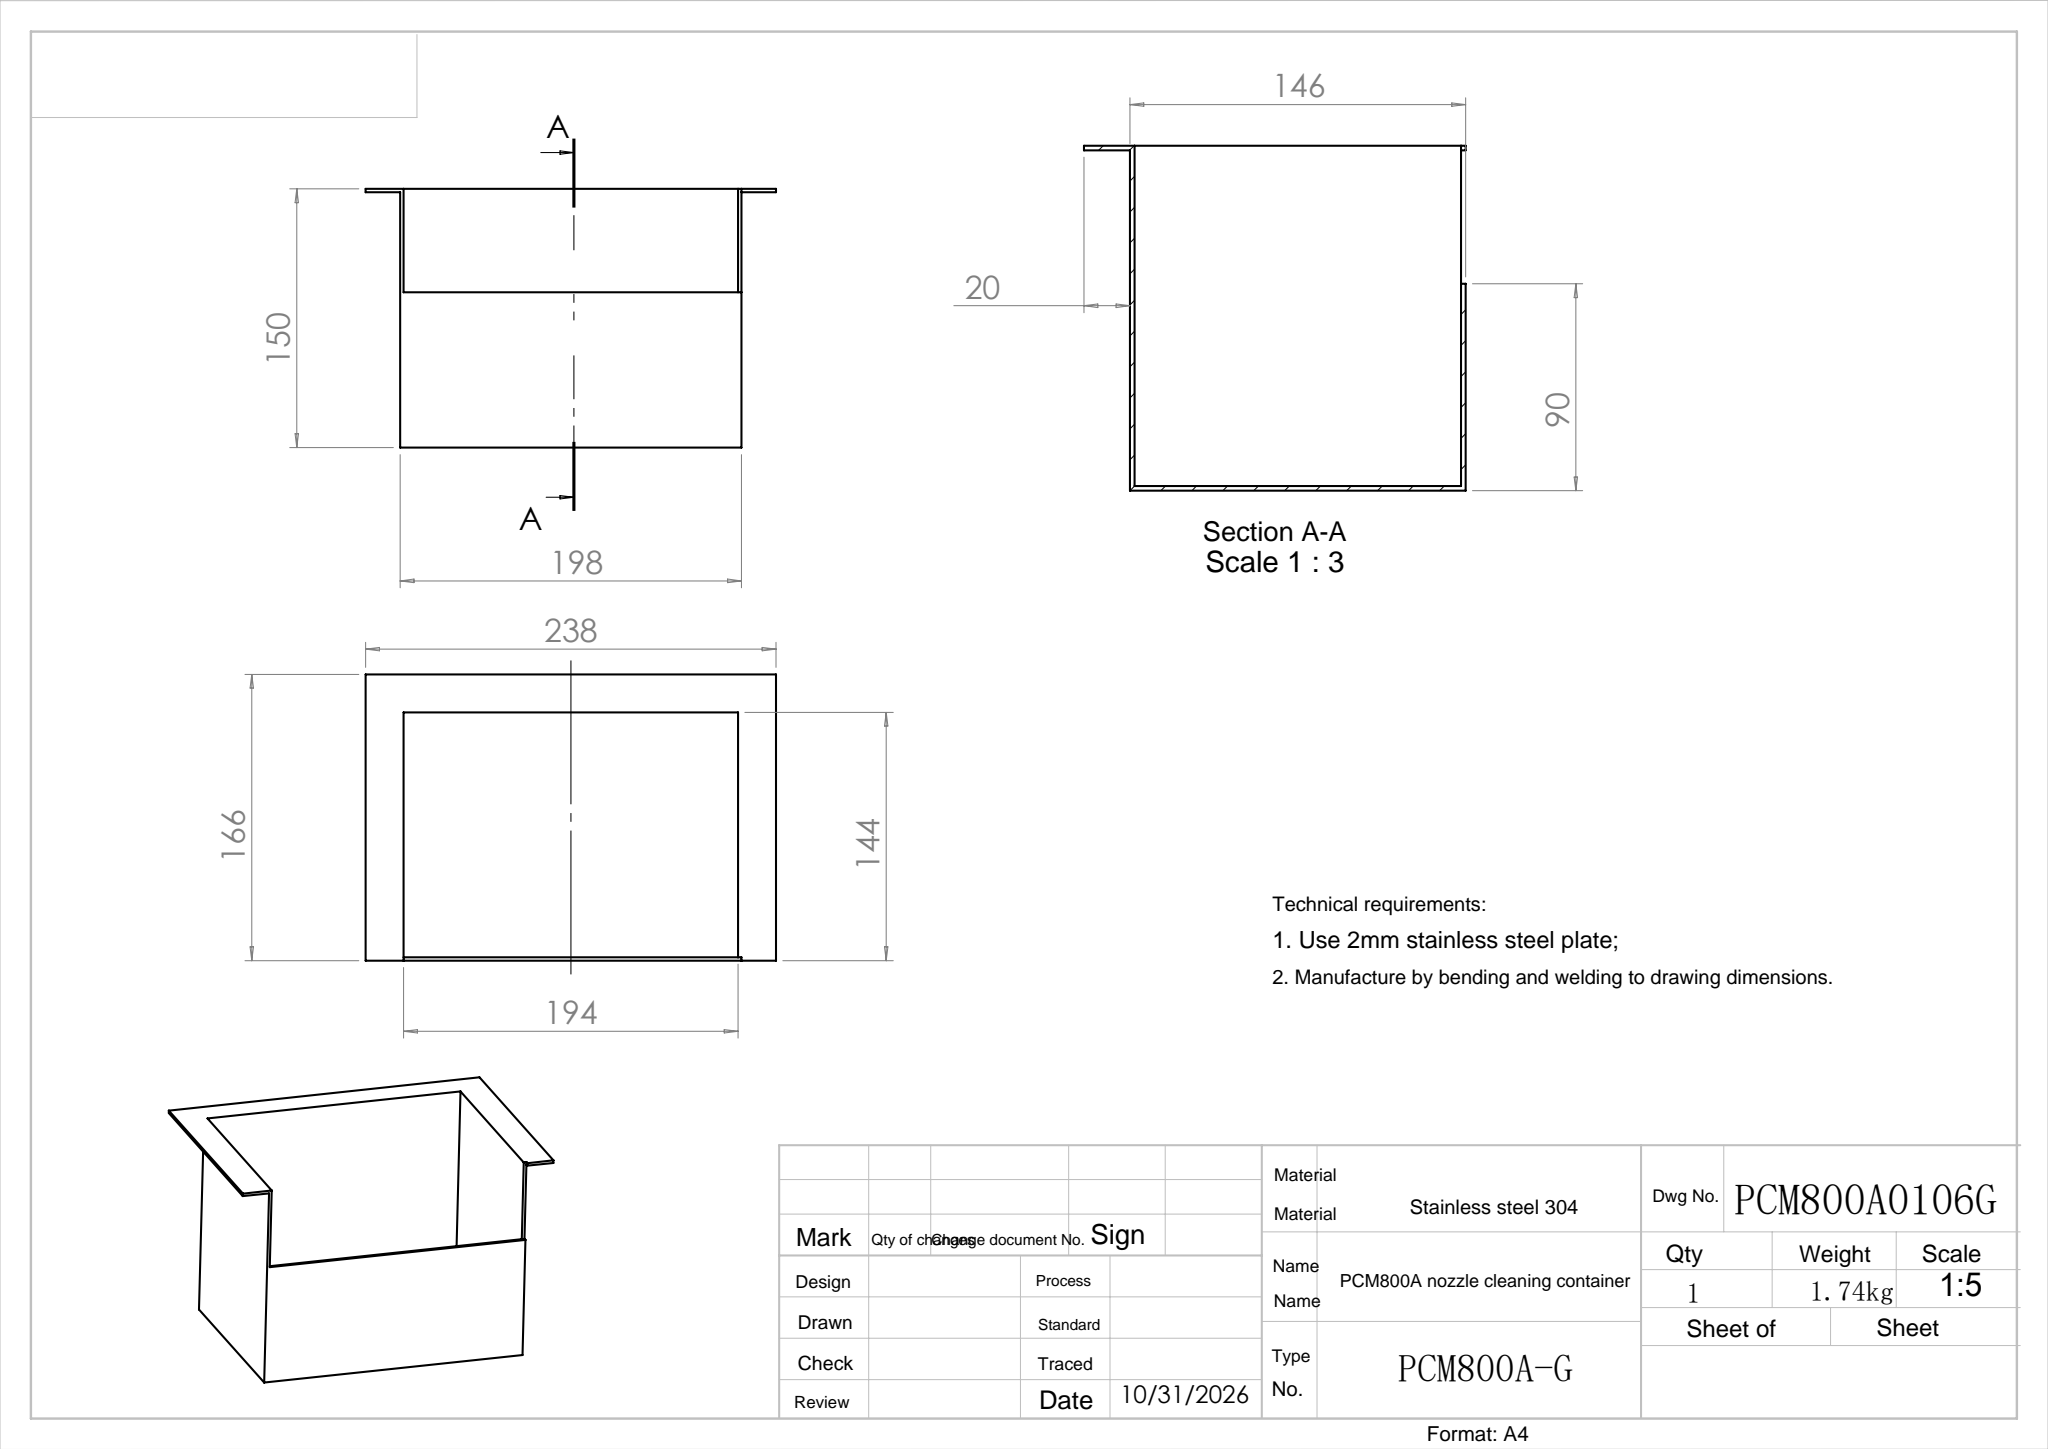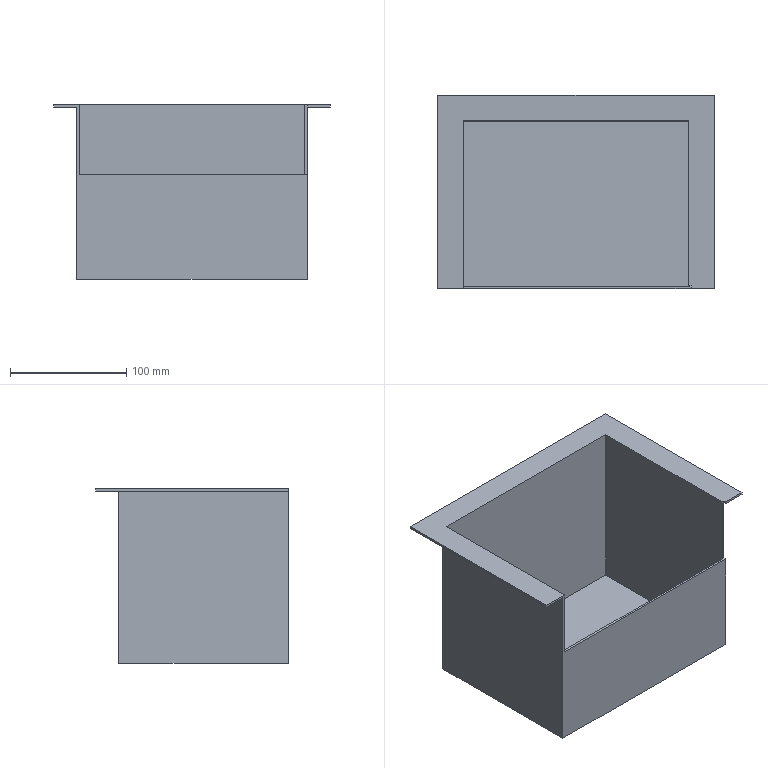Part | SolidWorks | features ICE 2, Extrusion 1, Shell 1 | 1 solid | 19 faces | box 238 x 166 x 150 mm | volume 256776 mm3 | plane 19
STEP:
#1=CARTESIAN_POINT('',(198.,-146.,150.));
#2=VERTEX_POINT('',#1);
#3=CARTESIAN_POINT('',(218.,-146.,150.));
#4=VERTEX_POINT('',#3);
#5=CARTESIAN_POINT('',(0.,-146.,150.));
#6=DIRECTION('',(1.,0.,0.));
#7=VECTOR('',#6,1000.);
#8=LINE('',#5,#7);
#9=EDGE_CURVE('',#2,#4,#8,.T.);
#10=ORIENTED_EDGE('',*,*,#9,.F.);
#11=CARTESIAN_POINT('',(198.,-146.,148.));
#12=VERTEX_POINT('',#11);
#13=CARTESIAN_POINT('',(198.,-146.,150.));
#14=DIRECTION('',(0.,0.,1.));
#15=VECTOR('',#14,1000.);
#16=LINE('',#13,#15);
#17=EDGE_CURVE('',#12,#2,#16,.T.);
#18=ORIENTED_EDGE('',*,*,#17,.F.);
#19=CARTESIAN_POINT('',(218.,-146.,148.));
#20=VERTEX_POINT('',#19);
#21=CARTESIAN_POINT('',(198.,-146.,148.));
#22=DIRECTION('',(1.,0.,0.));
#23=VECTOR('',#22,1000.);
#24=LINE('',#21,#23);
#25=EDGE_CURVE('',#12,#20,#24,.T.);
#26=ORIENTED_EDGE('',*,*,#25,.T.);
#27=CARTESIAN_POINT('',(218.,-146.,148.));
#28=DIRECTION('',(0.,0.,1.));
#29=VECTOR('',#28,1000.);
#30=LINE('',#27,#29);
#31=EDGE_CURVE('',#20,#4,#30,.T.);
#32=ORIENTED_EDGE('',*,*,#31,.T.);
#33=EDGE_LOOP('',(#10,#18,#26,#32));
#34=FACE_OUTER_BOUND('',#33,.T.);
#35=CARTESIAN_POINT('',(0.,-146.,150.));
#36=DIRECTION('',(0.,1.,0.));
#37=DIRECTION('',(0.,0.,1.));
#38=AXIS2_PLACEMENT_3D('',#35,#36,#37);
#39=PLANE('',#38);
#40=ADVANCED_FACE('',(#34),#39,.F.);
#41=CARTESIAN_POINT('',(0.,-146.,148.));
#42=VERTEX_POINT('',#41);
#43=CARTESIAN_POINT('',(0.,0.,148.));
#44=VERTEX_POINT('',#43);
#45=CARTESIAN_POINT('',(0.,0.,148.));
#46=DIRECTION('',(0.,1.,0.));
#47=VECTOR('',#46,1000.);
#48=LINE('',#45,#47);
#49=EDGE_CURVE('',#42,#44,#48,.T.);
#50=ORIENTED_EDGE('',*,*,#49,.T.);
#51=CARTESIAN_POINT('',(0.,0.,0.));
#52=VERTEX_POINT('',#51);
#53=CARTESIAN_POINT('',(0.,0.,150.));
#54=DIRECTION('',(0.,0.,-1.));
#55=VECTOR('',#54,1000.);
#56=LINE('',#53,#55);
#57=EDGE_CURVE('',#44,#52,#56,.T.);
#58=ORIENTED_EDGE('',*,*,#57,.T.);
#59=CARTESIAN_POINT('',(0.,-146.,0.));
#60=VERTEX_POINT('',#59);
#61=CARTESIAN_POINT('',(0.,0.,0.));
#62=DIRECTION('',(0.,-1.,0.));
#63=VECTOR('',#62,1000.);
#64=LINE('',#61,#63);
#65=EDGE_CURVE('',#52,#60,#64,.T.);
#66=ORIENTED_EDGE('',*,*,#65,.T.);
#67=CARTESIAN_POINT('',(0.,-146.,150.));
#68=DIRECTION('',(0.,0.,-1.));
#69=VECTOR('',#68,1000.);
#70=LINE('',#67,#69);
#71=EDGE_CURVE('',#42,#60,#70,.T.);
#72=ORIENTED_EDGE('',*,*,#71,.F.);
#73=EDGE_LOOP('',(#50,#58,#66,#72));
#74=FACE_OUTER_BOUND('',#73,.T.);
#75=CARTESIAN_POINT('',(0.,0.,150.));
#76=DIRECTION('',(1.,0.,0.));
#77=DIRECTION('',(0.,1.,0.));
#78=AXIS2_PLACEMENT_3D('',#75,#76,#77);
#79=PLANE('',#78);
#80=ADVANCED_FACE('',(#74),#79,.F.);
#81=CARTESIAN_POINT('',(198.,-144.,90.));
#82=VERTEX_POINT('',#81);
#83=CARTESIAN_POINT('',(198.,-144.,148.));
#84=VERTEX_POINT('',#83);
#85=CARTESIAN_POINT('',(198.,-144.,150.));
#86=DIRECTION('',(0.,0.,1.));
#87=VECTOR('',#86,1000.);
#88=LINE('',#85,#87);
#89=EDGE_CURVE('',#82,#84,#88,.T.);
#90=ORIENTED_EDGE('',*,*,#89,.F.);
#91=CARTESIAN_POINT('',(198.,-146.,90.));
#92=VERTEX_POINT('',#91);
#93=CARTESIAN_POINT('',(198.,-144.,90.));
#94=DIRECTION('',(0.,-1.,0.));
#95=VECTOR('',#94,1000.);
#96=LINE('',#93,#95);
#97=EDGE_CURVE('',#82,#92,#96,.T.);
#98=ORIENTED_EDGE('',*,*,#97,.T.);
#99=CARTESIAN_POINT('',(198.,-146.,0.));
#100=VERTEX_POINT('',#99);
#101=CARTESIAN_POINT('',(198.,-146.,150.));
#102=DIRECTION('',(0.,0.,-1.));
#103=VECTOR('',#102,1000.);
#104=LINE('',#101,#103);
#105=EDGE_CURVE('',#92,#100,#104,.T.);
#106=ORIENTED_EDGE('',*,*,#105,.T.);
#107=CARTESIAN_POINT('',(198.,0.,0.));
#108=VERTEX_POINT('',#107);
#109=CARTESIAN_POINT('',(198.,0.,0.));
#110=DIRECTION('',(0.,1.,0.));
#111=VECTOR('',#110,1000.);
#112=LINE('',#109,#111);
#113=EDGE_CURVE('',#100,#108,#112,.T.);
#114=ORIENTED_EDGE('',*,*,#113,.T.);
#115=CARTESIAN_POINT('',(198.,0.,148.));
#116=VERTEX_POINT('',#115);
#117=CARTESIAN_POINT('',(198.,0.,150.));
#118=DIRECTION('',(0.,0.,-1.));
#119=VECTOR('',#118,1000.);
#120=LINE('',#117,#119);
#121=EDGE_CURVE('',#116,#108,#120,.T.);
#122=ORIENTED_EDGE('',*,*,#121,.F.);
#123=CARTESIAN_POINT('',(198.,-146.,148.));
#124=DIRECTION('',(0.,-1.,0.));
#125=VECTOR('',#124,1000.);
#126=LINE('',#123,#125);
#127=EDGE_CURVE('',#116,#84,#126,.T.);
#128=ORIENTED_EDGE('',*,*,#127,.T.);
#129=EDGE_LOOP('',(#90,#98,#106,#114,#122,#128));
#130=FACE_OUTER_BOUND('',#129,.T.);
#131=CARTESIAN_POINT('',(198.,0.,150.));
#132=DIRECTION('',(-1.,0.,0.));
#133=DIRECTION('',(0.,-1.,0.));
#134=AXIS2_PLACEMENT_3D('',#131,#132,#133);
#135=PLANE('',#134);
#136=ADVANCED_FACE('',(#130),#135,.F.);
#137=CARTESIAN_POINT('',(198.,0.,148.));
#138=DIRECTION('',(1.,0.,0.));
#139=VECTOR('',#138,1000.);
#140=LINE('',#137,#139);
#141=EDGE_CURVE('',#44,#116,#140,.T.);
#142=ORIENTED_EDGE('',*,*,#141,.T.);
#143=ORIENTED_EDGE('',*,*,#121,.T.);
#144=CARTESIAN_POINT('',(0.,0.,0.));
#145=DIRECTION('',(-1.,0.,0.));
#146=VECTOR('',#145,1000.);
#147=LINE('',#144,#146);
#148=EDGE_CURVE('',#108,#52,#147,.T.);
#149=ORIENTED_EDGE('',*,*,#148,.T.);
#150=ORIENTED_EDGE('',*,*,#57,.F.);
#151=EDGE_LOOP('',(#142,#143,#149,#150));
#152=FACE_OUTER_BOUND('',#151,.T.);
#153=CARTESIAN_POINT('',(0.,0.,150.));
#154=DIRECTION('',(0.,-1.,0.));
#155=DIRECTION('',(0.,0.,-1.));
#156=AXIS2_PLACEMENT_3D('',#153,#154,#155);
#157=PLANE('',#156);
#158=ADVANCED_FACE('',(#152),#157,.F.);
#159=CARTESIAN_POINT('',(2.,-146.,90.));
#160=VERTEX_POINT('',#159);
#161=CARTESIAN_POINT('',(2.,-146.,90.));
#162=DIRECTION('',(1.,0.,0.));
#163=VECTOR('',#162,1000.);
#164=LINE('',#161,#163);
#165=EDGE_CURVE('',#160,#92,#164,.T.);
#166=ORIENTED_EDGE('',*,*,#165,.F.);
#167=CARTESIAN_POINT('',(2.,-146.,150.));
#168=VERTEX_POINT('',#167);
#169=CARTESIAN_POINT('',(2.,-146.,150.));
#170=DIRECTION('',(0.,0.,-1.));
#171=VECTOR('',#170,1000.);
#172=LINE('',#169,#171);
#173=EDGE_CURVE('',#168,#160,#172,.T.);
#174=ORIENTED_EDGE('',*,*,#173,.F.);
#175=CARTESIAN_POINT('',(-20.,-146.,150.));
#176=VERTEX_POINT('',#175);
#177=CARTESIAN_POINT('',(0.,-146.,150.));
#178=DIRECTION('',(1.,0.,0.));
#179=VECTOR('',#178,1000.);
#180=LINE('',#177,#179);
#181=EDGE_CURVE('',#176,#168,#180,.T.);
#182=ORIENTED_EDGE('',*,*,#181,.F.);
#183=CARTESIAN_POINT('',(-20.,-146.,148.));
#184=VERTEX_POINT('',#183);
#185=CARTESIAN_POINT('',(-20.,-146.,148.));
#186=DIRECTION('',(0.,0.,1.));
#187=VECTOR('',#186,1000.);
#188=LINE('',#185,#187);
#189=EDGE_CURVE('',#184,#176,#188,.T.);
#190=ORIENTED_EDGE('',*,*,#189,.F.);
#191=CARTESIAN_POINT('',(0.,-146.,148.));
#192=DIRECTION('',(1.,0.,0.));
#193=VECTOR('',#192,1000.);
#194=LINE('',#191,#193);
#195=EDGE_CURVE('',#184,#42,#194,.T.);
#196=ORIENTED_EDGE('',*,*,#195,.T.);
#197=ORIENTED_EDGE('',*,*,#71,.T.);
#198=CARTESIAN_POINT('',(0.,-146.,0.));
#199=DIRECTION('',(1.,0.,0.));
#200=VECTOR('',#199,1000.);
#201=LINE('',#198,#200);
#202=EDGE_CURVE('',#60,#100,#201,.T.);
#203=ORIENTED_EDGE('',*,*,#202,.T.);
#204=ORIENTED_EDGE('',*,*,#105,.F.);
#205=EDGE_LOOP('',(#166,#174,#182,#190,#196,#197,#203,#204));
#206=FACE_OUTER_BOUND('',#205,.T.);
#207=CARTESIAN_POINT('',(0.,-146.,150.));
#208=DIRECTION('',(0.,1.,0.));
#209=DIRECTION('',(0.,0.,1.));
#210=AXIS2_PLACEMENT_3D('',#207,#208,#209);
#211=PLANE('',#210);
#212=ADVANCED_FACE('',(#206),#211,.F.);
#213=ORIENTED_EDGE('',*,*,#181,.T.);
#214=CARTESIAN_POINT('',(2.,-2.,150.));
#215=VERTEX_POINT('',#214);
#216=CARTESIAN_POINT('',(2.,0.,150.));
#217=DIRECTION('',(0.,-1.,0.));
#218=VECTOR('',#217,1000.);
#219=LINE('',#216,#218);
#220=EDGE_CURVE('',#215,#168,#219,.T.);
#221=ORIENTED_EDGE('',*,*,#220,.F.);
#222=CARTESIAN_POINT('',(196.,-2.,150.));
#223=VERTEX_POINT('',#222);
#224=CARTESIAN_POINT('',(0.,-2.,150.));
#225=DIRECTION('',(-1.,0.,0.));
#226=VECTOR('',#225,1000.);
#227=LINE('',#224,#226);
#228=EDGE_CURVE('',#223,#215,#227,.T.);
#229=ORIENTED_EDGE('',*,*,#228,.F.);
#230=CARTESIAN_POINT('',(196.,-144.,150.));
#231=VERTEX_POINT('',#230);
#232=CARTESIAN_POINT('',(196.,0.,150.));
#233=DIRECTION('',(0.,1.,0.));
#234=VECTOR('',#233,1000.);
#235=LINE('',#232,#234);
#236=EDGE_CURVE('',#231,#223,#235,.T.);
#237=ORIENTED_EDGE('',*,*,#236,.F.);
#238=CARTESIAN_POINT('',(198.,-144.,150.));
#239=VERTEX_POINT('',#238);
#240=CARTESIAN_POINT('',(2.,-144.,150.));
#241=DIRECTION('',(-1.,0.,0.));
#242=VECTOR('',#241,1000.);
#243=LINE('',#240,#242);
#244=EDGE_CURVE('',#239,#231,#243,.T.);
#245=ORIENTED_EDGE('',*,*,#244,.F.);
#246=CARTESIAN_POINT('',(198.,-144.,150.));
#247=DIRECTION('',(0.,-1.,0.));
#248=VECTOR('',#247,1000.);
#249=LINE('',#246,#248);
#250=EDGE_CURVE('',#239,#2,#249,.T.);
#251=ORIENTED_EDGE('',*,*,#250,.T.);
#252=ORIENTED_EDGE('',*,*,#9,.T.);
#253=CARTESIAN_POINT('',(218.,20.,150.));
#254=VERTEX_POINT('',#253);
#255=CARTESIAN_POINT('',(218.,-146.,150.));
#256=DIRECTION('',(0.,1.,0.));
#257=VECTOR('',#256,1000.);
#258=LINE('',#255,#257);
#259=EDGE_CURVE('',#4,#254,#258,.T.);
#260=ORIENTED_EDGE('',*,*,#259,.T.);
#261=CARTESIAN_POINT('',(-20.,20.,150.));
#262=VERTEX_POINT('',#261);
#263=CARTESIAN_POINT('',(218.,20.,150.));
#264=DIRECTION('',(-1.,0.,0.));
#265=VECTOR('',#264,1000.);
#266=LINE('',#263,#265);
#267=EDGE_CURVE('',#254,#262,#266,.T.);
#268=ORIENTED_EDGE('',*,*,#267,.T.);
#269=CARTESIAN_POINT('',(-20.,20.,150.));
#270=DIRECTION('',(0.,-1.,0.));
#271=VECTOR('',#270,1000.);
#272=LINE('',#269,#271);
#273=EDGE_CURVE('',#262,#176,#272,.T.);
#274=ORIENTED_EDGE('',*,*,#273,.T.);
#275=EDGE_LOOP('',(#213,#221,#229,#237,#245,#251,#252,#260,#268,#274));
#276=FACE_OUTER_BOUND('',#275,.T.);
#277=CARTESIAN_POINT('',(0.,-146.,150.));
#278=DIRECTION('',(0.,0.,1.));
#279=DIRECTION('',(1.,0.,0.));
#280=AXIS2_PLACEMENT_3D('',#277,#278,#279);
#281=PLANE('',#280);
#282=ADVANCED_FACE('',(#276),#281,.T.);
#283=ORIENTED_EDGE('',*,*,#65,.F.);
#284=ORIENTED_EDGE('',*,*,#148,.F.);
#285=ORIENTED_EDGE('',*,*,#113,.F.);
#286=ORIENTED_EDGE('',*,*,#202,.F.);
#287=EDGE_LOOP('',(#283,#284,#285,#286));
#288=FACE_OUTER_BOUND('',#287,.T.);
#289=CARTESIAN_POINT('',(0.,-146.,0.));
#290=DIRECTION('',(0.,0.,1.));
#291=DIRECTION('',(1.,0.,0.));
#292=AXIS2_PLACEMENT_3D('',#289,#290,#291);
#293=PLANE('',#292);
#294=ADVANCED_FACE('',(#288),#293,.F.);
#295=CARTESIAN_POINT('',(2.,-2.,2.));
#296=VERTEX_POINT('',#295);
#297=CARTESIAN_POINT('',(2.,-144.,2.));
#298=VERTEX_POINT('',#297);
#299=CARTESIAN_POINT('',(2.,0.,2.));
#300=DIRECTION('',(0.,-1.,0.));
#301=VECTOR('',#300,1000.);
#302=LINE('',#299,#301);
#303=EDGE_CURVE('',#296,#298,#302,.T.);
#304=ORIENTED_EDGE('',*,*,#303,.F.);
#305=CARTESIAN_POINT('',(2.,-2.,150.));
#306=DIRECTION('',(0.,0.,-1.));
#307=VECTOR('',#306,1000.);
#308=LINE('',#305,#307);
#309=EDGE_CURVE('',#215,#296,#308,.T.);
#310=ORIENTED_EDGE('',*,*,#309,.F.);
#311=ORIENTED_EDGE('',*,*,#220,.T.);
#312=ORIENTED_EDGE('',*,*,#173,.T.);
#313=CARTESIAN_POINT('',(2.,-144.,90.));
#314=VERTEX_POINT('',#313);
#315=CARTESIAN_POINT('',(2.,-144.,90.));
#316=DIRECTION('',(0.,-1.,0.));
#317=VECTOR('',#316,1000.);
#318=LINE('',#315,#317);
#319=EDGE_CURVE('',#314,#160,#318,.T.);
#320=ORIENTED_EDGE('',*,*,#319,.F.);
#321=CARTESIAN_POINT('',(2.,-144.,150.));
#322=DIRECTION('',(0.,0.,-1.));
#323=VECTOR('',#322,1000.);
#324=LINE('',#321,#323);
#325=EDGE_CURVE('',#314,#298,#324,.T.);
#326=ORIENTED_EDGE('',*,*,#325,.T.);
#327=EDGE_LOOP('',(#304,#310,#311,#312,#320,#326));
#328=FACE_OUTER_BOUND('',#327,.T.);
#329=CARTESIAN_POINT('',(2.,0.,150.));
#330=DIRECTION('',(1.,0.,0.));
#331=DIRECTION('',(0.,1.,0.));
#332=AXIS2_PLACEMENT_3D('',#329,#330,#331);
#333=PLANE('',#332);
#334=ADVANCED_FACE('',(#328),#333,.T.);
#335=CARTESIAN_POINT('',(196.,-144.,90.));
#336=VERTEX_POINT('',#335);
#337=CARTESIAN_POINT('',(2.,-144.,90.));
#338=DIRECTION('',(1.,0.,0.));
#339=VECTOR('',#338,1000.);
#340=LINE('',#337,#339);
#341=EDGE_CURVE('',#314,#336,#340,.T.);
#342=ORIENTED_EDGE('',*,*,#341,.T.);
#343=CARTESIAN_POINT('',(196.,-144.,2.));
#344=VERTEX_POINT('',#343);
#345=CARTESIAN_POINT('',(196.,-144.,150.));
#346=DIRECTION('',(0.,0.,-1.));
#347=VECTOR('',#346,1000.);
#348=LINE('',#345,#347);
#349=EDGE_CURVE('',#336,#344,#348,.T.);
#350=ORIENTED_EDGE('',*,*,#349,.T.);
#351=CARTESIAN_POINT('',(0.,-144.,2.));
#352=DIRECTION('',(1.,0.,0.));
#353=VECTOR('',#352,1000.);
#354=LINE('',#351,#353);
#355=EDGE_CURVE('',#298,#344,#354,.T.);
#356=ORIENTED_EDGE('',*,*,#355,.F.);
#357=ORIENTED_EDGE('',*,*,#325,.F.);
#358=EDGE_LOOP('',(#342,#350,#356,#357));
#359=FACE_OUTER_BOUND('',#358,.T.);
#360=CARTESIAN_POINT('',(0.,-144.,150.));
#361=DIRECTION('',(0.,1.,0.));
#362=DIRECTION('',(0.,0.,1.));
#363=AXIS2_PLACEMENT_3D('',#360,#361,#362);
#364=PLANE('',#363);
#365=ADVANCED_FACE('',(#359),#364,.T.);
#366=CARTESIAN_POINT('',(196.,-2.,2.));
#367=VERTEX_POINT('',#366);
#368=CARTESIAN_POINT('',(196.,0.,2.));
#369=DIRECTION('',(0.,1.,0.));
#370=VECTOR('',#369,1000.);
#371=LINE('',#368,#370);
#372=EDGE_CURVE('',#344,#367,#371,.T.);
#373=ORIENTED_EDGE('',*,*,#372,.F.);
#374=ORIENTED_EDGE('',*,*,#349,.F.);
#375=CARTESIAN_POINT('',(196.,-144.,150.));
#376=DIRECTION('',(0.,0.,-1.));
#377=VECTOR('',#376,1000.);
#378=LINE('',#375,#377);
#379=EDGE_CURVE('',#231,#336,#378,.T.);
#380=ORIENTED_EDGE('',*,*,#379,.F.);
#381=ORIENTED_EDGE('',*,*,#236,.T.);
#382=CARTESIAN_POINT('',(196.,-2.,150.));
#383=DIRECTION('',(0.,0.,-1.));
#384=VECTOR('',#383,1000.);
#385=LINE('',#382,#384);
#386=EDGE_CURVE('',#223,#367,#385,.T.);
#387=ORIENTED_EDGE('',*,*,#386,.T.);
#388=EDGE_LOOP('',(#373,#374,#380,#381,#387));
#389=FACE_OUTER_BOUND('',#388,.T.);
#390=CARTESIAN_POINT('',(196.,0.,150.));
#391=DIRECTION('',(-1.,0.,0.));
#392=DIRECTION('',(0.,-1.,0.));
#393=AXIS2_PLACEMENT_3D('',#390,#391,#392);
#394=PLANE('',#393);
#395=ADVANCED_FACE('',(#389),#394,.T.);
#396=CARTESIAN_POINT('',(0.,-2.,2.));
#397=DIRECTION('',(-1.,0.,0.));
#398=VECTOR('',#397,1000.);
#399=LINE('',#396,#398);
#400=EDGE_CURVE('',#367,#296,#399,.T.);
#401=ORIENTED_EDGE('',*,*,#400,.F.);
#402=ORIENTED_EDGE('',*,*,#386,.F.);
#403=ORIENTED_EDGE('',*,*,#228,.T.);
#404=ORIENTED_EDGE('',*,*,#309,.T.);
#405=EDGE_LOOP('',(#401,#402,#403,#404));
#406=FACE_OUTER_BOUND('',#405,.T.);
#407=CARTESIAN_POINT('',(0.,-2.,150.));
#408=DIRECTION('',(0.,-1.,0.));
#409=DIRECTION('',(0.,0.,-1.));
#410=AXIS2_PLACEMENT_3D('',#407,#408,#409);
#411=PLANE('',#410);
#412=ADVANCED_FACE('',(#406),#411,.T.);
#413=ORIENTED_EDGE('',*,*,#303,.T.);
#414=ORIENTED_EDGE('',*,*,#355,.T.);
#415=ORIENTED_EDGE('',*,*,#372,.T.);
#416=ORIENTED_EDGE('',*,*,#400,.T.);
#417=EDGE_LOOP('',(#413,#414,#415,#416));
#418=FACE_OUTER_BOUND('',#417,.T.);
#419=CARTESIAN_POINT('',(0.,-146.,2.));
#420=DIRECTION('',(0.,0.,1.));
#421=DIRECTION('',(1.,0.,0.));
#422=AXIS2_PLACEMENT_3D('',#419,#420,#421);
#423=PLANE('',#422);
#424=ADVANCED_FACE('',(#418),#423,.T.);
#425=ORIENTED_EDGE('',*,*,#273,.F.);
#426=CARTESIAN_POINT('',(-20.,20.,148.));
#427=VERTEX_POINT('',#426);
#428=CARTESIAN_POINT('',(-20.,20.,148.));
#429=DIRECTION('',(0.,0.,1.));
#430=VECTOR('',#429,1000.);
#431=LINE('',#428,#430);
#432=EDGE_CURVE('',#427,#262,#431,.T.);
#433=ORIENTED_EDGE('',*,*,#432,.F.);
#434=CARTESIAN_POINT('',(-20.,20.,148.));
#435=DIRECTION('',(0.,-1.,0.));
#436=VECTOR('',#435,1000.);
#437=LINE('',#434,#436);
#438=EDGE_CURVE('',#427,#184,#437,.T.);
#439=ORIENTED_EDGE('',*,*,#438,.T.);
#440=ORIENTED_EDGE('',*,*,#189,.T.);
#441=EDGE_LOOP('',(#425,#433,#439,#440));
#442=FACE_OUTER_BOUND('',#441,.T.);
#443=CARTESIAN_POINT('',(-20.,20.,148.));
#444=DIRECTION('',(-1.,0.,0.));
#445=DIRECTION('',(0.,-1.,0.));
#446=AXIS2_PLACEMENT_3D('',#443,#444,#445);
#447=PLANE('',#446);
#448=ADVANCED_FACE('',(#442),#447,.T.);
#449=ORIENTED_EDGE('',*,*,#267,.F.);
#450=CARTESIAN_POINT('',(218.,20.,148.));
#451=VERTEX_POINT('',#450);
#452=CARTESIAN_POINT('',(218.,20.,148.));
#453=DIRECTION('',(0.,0.,1.));
#454=VECTOR('',#453,1000.);
#455=LINE('',#452,#454);
#456=EDGE_CURVE('',#451,#254,#455,.T.);
#457=ORIENTED_EDGE('',*,*,#456,.F.);
#458=CARTESIAN_POINT('',(218.,20.,148.));
#459=DIRECTION('',(-1.,0.,0.));
#460=VECTOR('',#459,1000.);
#461=LINE('',#458,#460);
#462=EDGE_CURVE('',#451,#427,#461,.T.);
#463=ORIENTED_EDGE('',*,*,#462,.T.);
#464=ORIENTED_EDGE('',*,*,#432,.T.);
#465=EDGE_LOOP('',(#449,#457,#463,#464));
#466=FACE_OUTER_BOUND('',#465,.T.);
#467=CARTESIAN_POINT('',(218.,20.,148.));
#468=DIRECTION('',(0.,1.,0.));
#469=DIRECTION('',(-1.,0.,0.));
#470=AXIS2_PLACEMENT_3D('',#467,#468,#469);
#471=PLANE('',#470);
#472=ADVANCED_FACE('',(#466),#471,.T.);
#473=ORIENTED_EDGE('',*,*,#259,.F.);
#474=ORIENTED_EDGE('',*,*,#31,.F.);
#475=CARTESIAN_POINT('',(218.,-146.,148.));
#476=DIRECTION('',(0.,1.,0.));
#477=VECTOR('',#476,1000.);
#478=LINE('',#475,#477);
#479=EDGE_CURVE('',#20,#451,#478,.T.);
#480=ORIENTED_EDGE('',*,*,#479,.T.);
#481=ORIENTED_EDGE('',*,*,#456,.T.);
#482=EDGE_LOOP('',(#473,#474,#480,#481));
#483=FACE_OUTER_BOUND('',#482,.T.);
#484=CARTESIAN_POINT('',(218.,-146.,148.));
#485=DIRECTION('',(1.,0.,0.));
#486=DIRECTION('',(0.,0.,-1.));
#487=AXIS2_PLACEMENT_3D('',#484,#485,#486);
#488=PLANE('',#487);
#489=ADVANCED_FACE('',(#483),#488,.T.);
#490=ORIENTED_EDGE('',*,*,#127,.F.);
#491=ORIENTED_EDGE('',*,*,#141,.F.);
#492=ORIENTED_EDGE('',*,*,#49,.F.);
#493=ORIENTED_EDGE('',*,*,#195,.F.);
#494=ORIENTED_EDGE('',*,*,#438,.F.);
#495=ORIENTED_EDGE('',*,*,#462,.F.);
#496=ORIENTED_EDGE('',*,*,#479,.F.);
#497=ORIENTED_EDGE('',*,*,#25,.F.);
#498=CARTESIAN_POINT('',(198.,-146.,148.));
#499=DIRECTION('',(0.,-1.,0.));
#500=VECTOR('',#499,1000.);
#501=LINE('',#498,#500);
#502=EDGE_CURVE('',#84,#12,#501,.T.);
#503=ORIENTED_EDGE('',*,*,#502,.F.);
#504=EDGE_LOOP('',(#490,#491,#492,#493,#494,#495,#496,#497,#503));
#505=FACE_OUTER_BOUND('',#504,.T.);
#506=CARTESIAN_POINT('',(198.,0.,148.));
#507=DIRECTION('',(0.,0.,1.));
#508=DIRECTION('',(1.,0.,0.));
#509=AXIS2_PLACEMENT_3D('',#506,#507,#508);
#510=PLANE('',#509);
#511=ADVANCED_FACE('',(#505),#510,.F.);
#512=ORIENTED_EDGE('',*,*,#17,.T.);
#513=ORIENTED_EDGE('',*,*,#250,.F.);
#514=CARTESIAN_POINT('',(198.,-144.,150.));
#515=DIRECTION('',(0.,0.,1.));
#516=VECTOR('',#515,1000.);
#517=LINE('',#514,#516);
#518=EDGE_CURVE('',#84,#239,#517,.T.);
#519=ORIENTED_EDGE('',*,*,#518,.F.);
#520=ORIENTED_EDGE('',*,*,#502,.T.);
#521=EDGE_LOOP('',(#512,#513,#519,#520));
#522=FACE_OUTER_BOUND('',#521,.T.);
#523=CARTESIAN_POINT('',(198.,-144.,150.));
#524=DIRECTION('',(1.,0.,0.));
#525=DIRECTION('',(0.,0.,-1.));
#526=AXIS2_PLACEMENT_3D('',#523,#524,#525);
#527=PLANE('',#526);
#528=ADVANCED_FACE('',(#522),#527,.F.);
#529=ORIENTED_EDGE('',*,*,#165,.T.);
#530=ORIENTED_EDGE('',*,*,#97,.F.);
#531=CARTESIAN_POINT('',(2.,-144.,90.));
#532=DIRECTION('',(1.,0.,0.));
#533=VECTOR('',#532,1000.);
#534=LINE('',#531,#533);
#535=EDGE_CURVE('',#336,#82,#534,.T.);
#536=ORIENTED_EDGE('',*,*,#535,.F.);
#537=ORIENTED_EDGE('',*,*,#341,.F.);
#538=ORIENTED_EDGE('',*,*,#319,.T.);
#539=EDGE_LOOP('',(#529,#530,#536,#537,#538));
#540=FACE_OUTER_BOUND('',#539,.T.);
#541=CARTESIAN_POINT('',(2.,-144.,90.));
#542=DIRECTION('',(0.,0.,-1.));
#543=DIRECTION('',(-1.,0.,0.));
#544=AXIS2_PLACEMENT_3D('',#541,#542,#543);
#545=PLANE('',#544);
#546=ADVANCED_FACE('',(#540),#545,.F.);
#547=ORIENTED_EDGE('',*,*,#535,.T.);
#548=ORIENTED_EDGE('',*,*,#89,.T.);
#549=ORIENTED_EDGE('',*,*,#518,.T.);
#550=ORIENTED_EDGE('',*,*,#244,.T.);
#551=ORIENTED_EDGE('',*,*,#379,.T.);
#552=EDGE_LOOP('',(#547,#548,#549,#550,#551));
#553=FACE_OUTER_BOUND('',#552,.T.);
#554=CARTESIAN_POINT('',(2.,-144.,90.));
#555=DIRECTION('',(0.,-1.,0.));
#556=DIRECTION('',(0.,0.,-1.));
#557=AXIS2_PLACEMENT_3D('',#554,#555,#556);
#558=PLANE('',#557);
#559=ADVANCED_FACE('',(#553),#558,.T.);
#560=CLOSED_SHELL('',(#40,#80,#136,#158,#212,#282,#294,#334,#365,#395,#412,#424,#448,#472,#489,#511,#528,#546,#559));
#561=MANIFOLD_SOLID_BREP('',#560);
#562=CARTESIAN_POINT('',(0.,0.,0.));
#563=DIRECTION('',(0.,0.,1.));
#564=DIRECTION('',(1.,0.,0.));
#565=AXIS2_PLACEMENT_3D('',#562,#563,#564);
#566=(LENGTH_UNIT()NAMED_UNIT(*)SI_UNIT(.MILLI.,.METRE.));
#567=UNCERTAINTY_MEASURE_WITH_UNIT(LENGTH_MEASURE(0.00001),#566,'','');
#568=(NAMED_UNIT(*)PLANE_ANGLE_UNIT()SI_UNIT($,.RADIAN.));
#569=(NAMED_UNIT(*)SI_UNIT($,.STERADIAN.)SOLID_ANGLE_UNIT());
#570=(GEOMETRIC_REPRESENTATION_CONTEXT(3)GLOBAL_UNCERTAINTY_ASSIGNED_CONTEXT((#567))GLOBAL_UNIT_ASSIGNED_CONTEXT((#566,#568,#569))REPRESENTATION_CONTEXT('',''));
#571=ADVANCED_BREP_SHAPE_REPRESENTATION('',(#561,#565),#570);